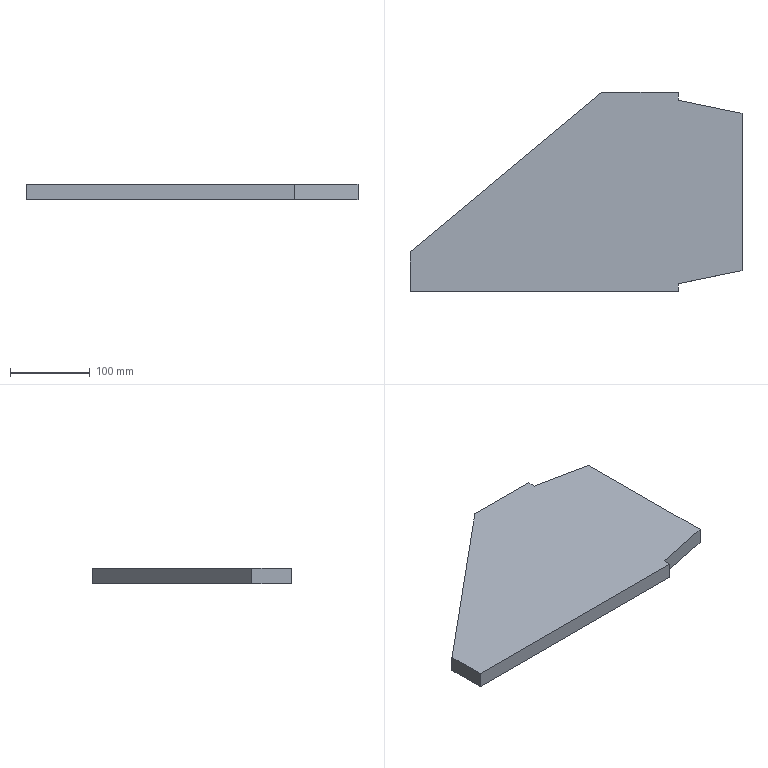Part | SolidWorks | features Extrusion 1 | 1 solid | 11 faces | box 416.402 x 250 x 20 mm | volume 1542694 mm3 | plane 11
STEP:
#1=CARTESIAN_POINT('',(15783.13,4614.36,0.));
#2=VERTEX_POINT('',#1);
#3=CARTESIAN_POINT('',(15783.13,4624.36,0.));
#4=VERTEX_POINT('',#3);
#5=CARTESIAN_POINT('',(15783.13,4614.36,0.));
#6=DIRECTION('',(0.,1.,0.));
#7=VECTOR('',#6,1000.);
#8=LINE('',#5,#7);
#9=EDGE_CURVE('',#2,#4,#8,.T.);
#10=ORIENTED_EDGE('',*,*,#9,.T.);
#11=CARTESIAN_POINT('',(15783.13,4624.36,20.));
#12=VERTEX_POINT('',#11);
#13=CARTESIAN_POINT('',(15783.13,4624.36,20.));
#14=DIRECTION('',(0.,0.,-1.));
#15=VECTOR('',#14,1000.);
#16=LINE('',#13,#15);
#17=EDGE_CURVE('',#12,#4,#16,.T.);
#18=ORIENTED_EDGE('',*,*,#17,.F.);
#19=CARTESIAN_POINT('',(15783.13,4614.36,20.));
#20=VERTEX_POINT('',#19);
#21=CARTESIAN_POINT('',(15783.13,4614.36,20.));
#22=DIRECTION('',(0.,1.,0.));
#23=VECTOR('',#22,1000.);
#24=LINE('',#21,#23);
#25=EDGE_CURVE('',#20,#12,#24,.T.);
#26=ORIENTED_EDGE('',*,*,#25,.F.);
#27=CARTESIAN_POINT('',(15783.13,4614.36,20.));
#28=DIRECTION('',(0.,0.,-1.));
#29=VECTOR('',#28,1000.);
#30=LINE('',#27,#29);
#31=EDGE_CURVE('',#20,#2,#30,.T.);
#32=ORIENTED_EDGE('',*,*,#31,.T.);
#33=EDGE_LOOP('',(#10,#18,#26,#32));
#34=FACE_OUTER_BOUND('',#33,.T.);
#35=CARTESIAN_POINT('',(15783.13,4614.36,20.));
#36=DIRECTION('',(-1.,0.,0.));
#37=DIRECTION('',(0.,0.,1.));
#38=AXIS2_PLACEMENT_3D('',#35,#36,#37);
#39=PLANE('',#38);
#40=ADVANCED_FACE('',(#34),#39,.F.);
#41=CARTESIAN_POINT('',(15687.257,4624.36,0.));
#42=VERTEX_POINT('',#41);
#43=CARTESIAN_POINT('',(15783.13,4624.36,0.));
#44=DIRECTION('',(-1.,0.,0.));
#45=VECTOR('',#44,1000.);
#46=LINE('',#43,#45);
#47=EDGE_CURVE('',#4,#42,#46,.T.);
#48=ORIENTED_EDGE('',*,*,#47,.T.);
#49=CARTESIAN_POINT('',(15687.257,4624.36,20.));
#50=VERTEX_POINT('',#49);
#51=CARTESIAN_POINT('',(15687.257,4624.36,20.));
#52=DIRECTION('',(0.,0.,-1.));
#53=VECTOR('',#52,1000.);
#54=LINE('',#51,#53);
#55=EDGE_CURVE('',#50,#42,#54,.T.);
#56=ORIENTED_EDGE('',*,*,#55,.F.);
#57=CARTESIAN_POINT('',(15783.13,4624.36,20.));
#58=DIRECTION('',(-1.,0.,0.));
#59=VECTOR('',#58,1000.);
#60=LINE('',#57,#59);
#61=EDGE_CURVE('',#12,#50,#60,.T.);
#62=ORIENTED_EDGE('',*,*,#61,.F.);
#63=ORIENTED_EDGE('',*,*,#17,.T.);
#64=EDGE_LOOP('',(#48,#56,#62,#63));
#65=FACE_OUTER_BOUND('',#64,.T.);
#66=CARTESIAN_POINT('',(15783.13,4624.36,20.));
#67=DIRECTION('',(0.,-1.,0.));
#68=DIRECTION('',(0.,0.,-1.));
#69=AXIS2_PLACEMENT_3D('',#66,#67,#68);
#70=PLANE('',#69);
#71=ADVANCED_FACE('',(#65),#70,.F.);
#72=CARTESIAN_POINT('',(15446.728,4424.36,0.));
#73=VERTEX_POINT('',#72);
#74=CARTESIAN_POINT('',(15687.257,4624.36,0.));
#75=DIRECTION('',(-0.7689,-0.6394,0.));
#76=VECTOR('',#75,1000.);
#77=LINE('',#74,#76);
#78=EDGE_CURVE('',#42,#73,#77,.T.);
#79=ORIENTED_EDGE('',*,*,#78,.T.);
#80=CARTESIAN_POINT('',(15446.728,4424.36,20.));
#81=VERTEX_POINT('',#80);
#82=CARTESIAN_POINT('',(15446.728,4424.36,20.));
#83=DIRECTION('',(0.,0.,-1.));
#84=VECTOR('',#83,1000.);
#85=LINE('',#82,#84);
#86=EDGE_CURVE('',#81,#73,#85,.T.);
#87=ORIENTED_EDGE('',*,*,#86,.F.);
#88=CARTESIAN_POINT('',(15687.257,4624.36,20.));
#89=DIRECTION('',(-0.7689,-0.6394,0.));
#90=VECTOR('',#89,1000.);
#91=LINE('',#88,#90);
#92=EDGE_CURVE('',#50,#81,#91,.T.);
#93=ORIENTED_EDGE('',*,*,#92,.F.);
#94=ORIENTED_EDGE('',*,*,#55,.T.);
#95=EDGE_LOOP('',(#79,#87,#93,#94));
#96=FACE_OUTER_BOUND('',#95,.T.);
#97=CARTESIAN_POINT('',(15687.257,4624.36,20.));
#98=DIRECTION('',(0.6394,-0.7689,0.));
#99=DIRECTION('',(0.7689,0.6394,0.));
#100=AXIS2_PLACEMENT_3D('',#97,#98,#99);
#101=PLANE('',#100);
#102=ADVANCED_FACE('',(#96),#101,.F.);
#103=CARTESIAN_POINT('',(15446.728,4374.36,0.));
#104=VERTEX_POINT('',#103);
#105=CARTESIAN_POINT('',(15446.728,4374.36,0.));
#106=DIRECTION('',(0.,-1.,0.));
#107=VECTOR('',#106,1000.);
#108=LINE('',#105,#107);
#109=EDGE_CURVE('',#73,#104,#108,.T.);
#110=ORIENTED_EDGE('',*,*,#109,.T.);
#111=CARTESIAN_POINT('',(15446.728,4374.36,20.));
#112=VERTEX_POINT('',#111);
#113=CARTESIAN_POINT('',(15446.728,4374.36,20.));
#114=DIRECTION('',(0.,0.,-1.));
#115=VECTOR('',#114,1000.);
#116=LINE('',#113,#115);
#117=EDGE_CURVE('',#112,#104,#116,.T.);
#118=ORIENTED_EDGE('',*,*,#117,.F.);
#119=CARTESIAN_POINT('',(15446.728,4374.36,20.));
#120=DIRECTION('',(0.,-1.,0.));
#121=VECTOR('',#120,1000.);
#122=LINE('',#119,#121);
#123=EDGE_CURVE('',#81,#112,#122,.T.);
#124=ORIENTED_EDGE('',*,*,#123,.F.);
#125=ORIENTED_EDGE('',*,*,#86,.T.);
#126=EDGE_LOOP('',(#110,#118,#124,#125));
#127=FACE_OUTER_BOUND('',#126,.T.);
#128=CARTESIAN_POINT('',(15446.728,4374.36,20.));
#129=DIRECTION('',(1.,0.,0.));
#130=DIRECTION('',(0.,0.,-1.));
#131=AXIS2_PLACEMENT_3D('',#128,#129,#130);
#132=PLANE('',#131);
#133=ADVANCED_FACE('',(#127),#132,.F.);
#134=CARTESIAN_POINT('',(15783.13,4374.36,0.));
#135=VERTEX_POINT('',#134);
#136=CARTESIAN_POINT('',(15446.728,4374.36,0.));
#137=DIRECTION('',(1.,0.,0.));
#138=VECTOR('',#137,1000.);
#139=LINE('',#136,#138);
#140=EDGE_CURVE('',#104,#135,#139,.T.);
#141=ORIENTED_EDGE('',*,*,#140,.T.);
#142=CARTESIAN_POINT('',(15783.13,4374.36,20.));
#143=VERTEX_POINT('',#142);
#144=CARTESIAN_POINT('',(15783.13,4374.36,20.));
#145=DIRECTION('',(0.,0.,-1.));
#146=VECTOR('',#145,1000.);
#147=LINE('',#144,#146);
#148=EDGE_CURVE('',#143,#135,#147,.T.);
#149=ORIENTED_EDGE('',*,*,#148,.F.);
#150=CARTESIAN_POINT('',(15446.728,4374.36,20.));
#151=DIRECTION('',(1.,0.,0.));
#152=VECTOR('',#151,1000.);
#153=LINE('',#150,#152);
#154=EDGE_CURVE('',#112,#143,#153,.T.);
#155=ORIENTED_EDGE('',*,*,#154,.F.);
#156=ORIENTED_EDGE('',*,*,#117,.T.);
#157=EDGE_LOOP('',(#141,#149,#155,#156));
#158=FACE_OUTER_BOUND('',#157,.T.);
#159=CARTESIAN_POINT('',(15446.728,4374.36,20.));
#160=DIRECTION('',(0.,1.,0.));
#161=DIRECTION('',(0.,0.,1.));
#162=AXIS2_PLACEMENT_3D('',#159,#160,#161);
#163=PLANE('',#162);
#164=ADVANCED_FACE('',(#158),#163,.F.);
#165=CARTESIAN_POINT('',(15783.13,4384.36,0.));
#166=VERTEX_POINT('',#165);
#167=CARTESIAN_POINT('',(15783.13,4384.36,0.));
#168=DIRECTION('',(0.,1.,0.));
#169=VECTOR('',#168,1000.);
#170=LINE('',#167,#169);
#171=EDGE_CURVE('',#135,#166,#170,.T.);
#172=ORIENTED_EDGE('',*,*,#171,.T.);
#173=CARTESIAN_POINT('',(15783.13,4384.36,20.));
#174=VERTEX_POINT('',#173);
#175=CARTESIAN_POINT('',(15783.13,4384.36,20.));
#176=DIRECTION('',(0.,0.,-1.));
#177=VECTOR('',#176,1000.);
#178=LINE('',#175,#177);
#179=EDGE_CURVE('',#174,#166,#178,.T.);
#180=ORIENTED_EDGE('',*,*,#179,.F.);
#181=CARTESIAN_POINT('',(15783.13,4384.36,20.));
#182=DIRECTION('',(0.,1.,0.));
#183=VECTOR('',#182,1000.);
#184=LINE('',#181,#183);
#185=EDGE_CURVE('',#143,#174,#184,.T.);
#186=ORIENTED_EDGE('',*,*,#185,.F.);
#187=ORIENTED_EDGE('',*,*,#148,.T.);
#188=EDGE_LOOP('',(#172,#180,#186,#187));
#189=FACE_OUTER_BOUND('',#188,.T.);
#190=CARTESIAN_POINT('',(15783.13,4384.36,20.));
#191=DIRECTION('',(-1.,0.,0.));
#192=DIRECTION('',(0.,0.,1.));
#193=AXIS2_PLACEMENT_3D('',#190,#191,#192);
#194=PLANE('',#193);
#195=ADVANCED_FACE('',(#189),#194,.F.);
#196=CARTESIAN_POINT('',(15863.13,4400.77,0.));
#197=VERTEX_POINT('',#196);
#198=CARTESIAN_POINT('',(15783.13,4384.36,0.));
#199=DIRECTION('',(0.9796,0.2009,0.));
#200=VECTOR('',#199,1000.);
#201=LINE('',#198,#200);
#202=EDGE_CURVE('',#166,#197,#201,.T.);
#203=ORIENTED_EDGE('',*,*,#202,.T.);
#204=CARTESIAN_POINT('',(15863.13,4400.77,20.));
#205=VERTEX_POINT('',#204);
#206=CARTESIAN_POINT('',(15863.13,4400.77,20.));
#207=DIRECTION('',(0.,0.,-1.));
#208=VECTOR('',#207,1000.);
#209=LINE('',#206,#208);
#210=EDGE_CURVE('',#205,#197,#209,.T.);
#211=ORIENTED_EDGE('',*,*,#210,.F.);
#212=CARTESIAN_POINT('',(15783.13,4384.36,20.));
#213=DIRECTION('',(0.9796,0.2009,0.));
#214=VECTOR('',#213,1000.);
#215=LINE('',#212,#214);
#216=EDGE_CURVE('',#174,#205,#215,.T.);
#217=ORIENTED_EDGE('',*,*,#216,.F.);
#218=ORIENTED_EDGE('',*,*,#179,.T.);
#219=EDGE_LOOP('',(#203,#211,#217,#218));
#220=FACE_OUTER_BOUND('',#219,.T.);
#221=CARTESIAN_POINT('',(15783.13,4384.36,20.));
#222=DIRECTION('',(-0.2009,0.9796,0.));
#223=DIRECTION('',(-0.9796,-0.2009,0.));
#224=AXIS2_PLACEMENT_3D('',#221,#222,#223);
#225=PLANE('',#224);
#226=ADVANCED_FACE('',(#220),#225,.F.);
#227=CARTESIAN_POINT('',(15863.13,4597.95,0.));
#228=VERTEX_POINT('',#227);
#229=CARTESIAN_POINT('',(15863.13,4597.95,0.));
#230=DIRECTION('',(0.,1.,0.));
#231=VECTOR('',#230,1000.);
#232=LINE('',#229,#231);
#233=EDGE_CURVE('',#197,#228,#232,.T.);
#234=ORIENTED_EDGE('',*,*,#233,.T.);
#235=CARTESIAN_POINT('',(15863.13,4597.95,20.));
#236=VERTEX_POINT('',#235);
#237=CARTESIAN_POINT('',(15863.13,4597.95,20.));
#238=DIRECTION('',(0.,0.,-1.));
#239=VECTOR('',#238,1000.);
#240=LINE('',#237,#239);
#241=EDGE_CURVE('',#236,#228,#240,.T.);
#242=ORIENTED_EDGE('',*,*,#241,.F.);
#243=CARTESIAN_POINT('',(15863.13,4597.95,20.));
#244=DIRECTION('',(0.,1.,0.));
#245=VECTOR('',#244,1000.);
#246=LINE('',#243,#245);
#247=EDGE_CURVE('',#205,#236,#246,.T.);
#248=ORIENTED_EDGE('',*,*,#247,.F.);
#249=ORIENTED_EDGE('',*,*,#210,.T.);
#250=EDGE_LOOP('',(#234,#242,#248,#249));
#251=FACE_OUTER_BOUND('',#250,.T.);
#252=CARTESIAN_POINT('',(15863.13,4597.95,20.));
#253=DIRECTION('',(-1.,0.,0.));
#254=DIRECTION('',(0.,0.,1.));
#255=AXIS2_PLACEMENT_3D('',#252,#253,#254);
#256=PLANE('',#255);
#257=ADVANCED_FACE('',(#251),#256,.F.);
#258=CARTESIAN_POINT('',(15783.13,4614.36,0.));
#259=DIRECTION('',(-0.9796,0.2009,0.));
#260=VECTOR('',#259,1000.);
#261=LINE('',#258,#260);
#262=EDGE_CURVE('',#228,#2,#261,.T.);
#263=ORIENTED_EDGE('',*,*,#262,.T.);
#264=ORIENTED_EDGE('',*,*,#31,.F.);
#265=CARTESIAN_POINT('',(15783.13,4614.36,20.));
#266=DIRECTION('',(-0.9796,0.2009,0.));
#267=VECTOR('',#266,1000.);
#268=LINE('',#265,#267);
#269=EDGE_CURVE('',#236,#20,#268,.T.);
#270=ORIENTED_EDGE('',*,*,#269,.F.);
#271=ORIENTED_EDGE('',*,*,#241,.T.);
#272=EDGE_LOOP('',(#263,#264,#270,#271));
#273=FACE_OUTER_BOUND('',#272,.T.);
#274=CARTESIAN_POINT('',(15783.13,4614.36,20.));
#275=DIRECTION('',(-0.2009,-0.9796,0.));
#276=DIRECTION('',(0.9796,-0.2009,0.));
#277=AXIS2_PLACEMENT_3D('',#274,#275,#276);
#278=PLANE('',#277);
#279=ADVANCED_FACE('',(#273),#278,.F.);
#280=ORIENTED_EDGE('',*,*,#25,.T.);
#281=ORIENTED_EDGE('',*,*,#61,.T.);
#282=ORIENTED_EDGE('',*,*,#92,.T.);
#283=ORIENTED_EDGE('',*,*,#123,.T.);
#284=ORIENTED_EDGE('',*,*,#154,.T.);
#285=ORIENTED_EDGE('',*,*,#185,.T.);
#286=ORIENTED_EDGE('',*,*,#216,.T.);
#287=ORIENTED_EDGE('',*,*,#247,.T.);
#288=ORIENTED_EDGE('',*,*,#269,.T.);
#289=EDGE_LOOP('',(#280,#281,#282,#283,#284,#285,#286,#287,#288));
#290=FACE_OUTER_BOUND('',#289,.T.);
#291=CARTESIAN_POINT('',(0.,0.,20.));
#292=DIRECTION('',(0.,0.,1.));
#293=DIRECTION('',(1.,0.,0.));
#294=AXIS2_PLACEMENT_3D('',#291,#292,#293);
#295=PLANE('',#294);
#296=ADVANCED_FACE('',(#290),#295,.T.);
#297=ORIENTED_EDGE('',*,*,#9,.F.);
#298=ORIENTED_EDGE('',*,*,#262,.F.);
#299=ORIENTED_EDGE('',*,*,#233,.F.);
#300=ORIENTED_EDGE('',*,*,#202,.F.);
#301=ORIENTED_EDGE('',*,*,#171,.F.);
#302=ORIENTED_EDGE('',*,*,#140,.F.);
#303=ORIENTED_EDGE('',*,*,#109,.F.);
#304=ORIENTED_EDGE('',*,*,#78,.F.);
#305=ORIENTED_EDGE('',*,*,#47,.F.);
#306=EDGE_LOOP('',(#297,#298,#299,#300,#301,#302,#303,#304,#305));
#307=FACE_OUTER_BOUND('',#306,.T.);
#308=CARTESIAN_POINT('',(0.,0.,0.));
#309=DIRECTION('',(0.,0.,1.));
#310=DIRECTION('',(1.,0.,0.));
#311=AXIS2_PLACEMENT_3D('',#308,#309,#310);
#312=PLANE('',#311);
#313=ADVANCED_FACE('',(#307),#312,.F.);
#314=CLOSED_SHELL('',(#40,#71,#102,#133,#164,#195,#226,#257,#279,#296,#313));
#315=MANIFOLD_SOLID_BREP('',#314);
#316=CARTESIAN_POINT('',(0.,0.,0.));
#317=DIRECTION('',(0.,0.,1.));
#318=DIRECTION('',(1.,0.,0.));
#319=AXIS2_PLACEMENT_3D('',#316,#317,#318);
#320=(LENGTH_UNIT()NAMED_UNIT(*)SI_UNIT(.MILLI.,.METRE.));
#321=UNCERTAINTY_MEASURE_WITH_UNIT(LENGTH_MEASURE(0.00001),#320,'','');
#322=(NAMED_UNIT(*)PLANE_ANGLE_UNIT()SI_UNIT($,.RADIAN.));
#323=(NAMED_UNIT(*)SI_UNIT($,.STERADIAN.)SOLID_ANGLE_UNIT());
#324=(GEOMETRIC_REPRESENTATION_CONTEXT(3)GLOBAL_UNCERTAINTY_ASSIGNED_CONTEXT((#321))GLOBAL_UNIT_ASSIGNED_CONTEXT((#320,#322,#323))REPRESENTATION_CONTEXT('',''));
#325=ADVANCED_BREP_SHAPE_REPRESENTATION('',(#315,#319),#324);